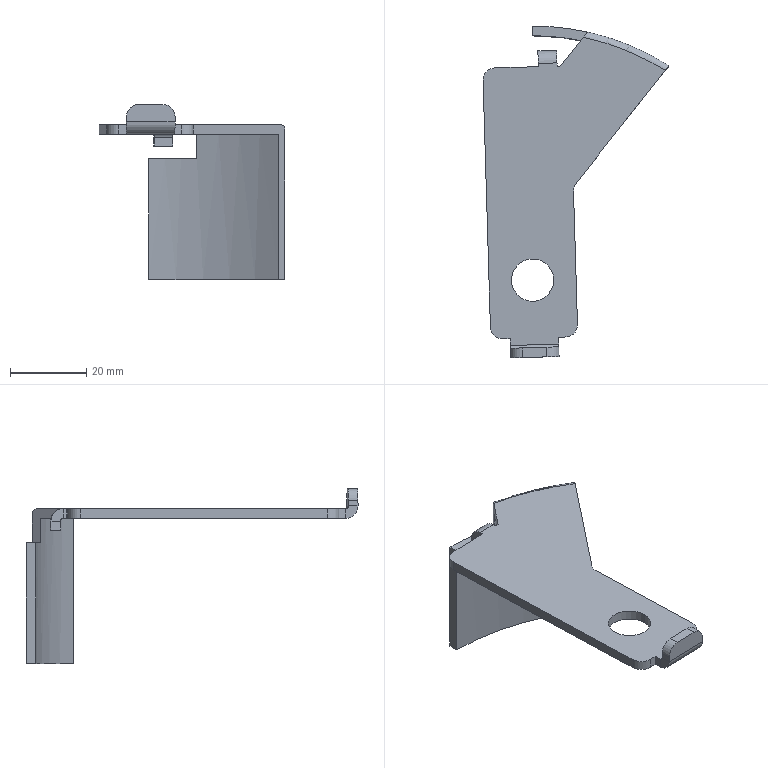Part | SolidWorks | features Fillet 2, ICE 2, SM3dBend 2, FlatPattern 1, SMBaseFlange 1, SheetMetal 1 | 1 solid | 47 faces | box 48.773 x 87.122 x 45.946 mm | volume 8989 mm3 | plane 31 | cylinder 15 | torus 1 | commonest cylinder face diameters 6.35 x7 1.473 x2 6.553 x2 11.112 x2 128.27 x1 133.35 x1
STEP:
#1=CARTESIAN_POINT('',(21.933,-23.71,2.54));
#2=VERTEX_POINT('',#1);
#3=CARTESIAN_POINT('',(21.935,-23.805,2.54));
#4=VERTEX_POINT('',#3);
#5=CARTESIAN_POINT('',(25.108,-23.71,2.54));
#6=DIRECTION('',(0.,0.,1.));
#7=DIRECTION('',(1.,0.,0.));
#8=AXIS2_PLACEMENT_3D('',#5,#6,#7);
#9=CIRCLE('',#8,3.175);
#10=EDGE_CURVE('',#2,#4,#9,.T.);
#11=ORIENTED_EDGE('',*,*,#10,.F.);
#12=CARTESIAN_POINT('',(21.933,-23.71,0.));
#13=VERTEX_POINT('',#12);
#14=CARTESIAN_POINT('',(21.933,-23.71,2.54));
#15=DIRECTION('',(0.,0.,-1.));
#16=VECTOR('',#15,1000.);
#17=LINE('',#14,#16);
#18=EDGE_CURVE('',#2,#13,#17,.T.);
#19=ORIENTED_EDGE('',*,*,#18,.T.);
#20=CARTESIAN_POINT('',(21.935,-23.805,0.));
#21=VERTEX_POINT('',#20);
#22=CARTESIAN_POINT('',(25.108,-23.71,0.));
#23=DIRECTION('',(0.,0.,-1.));
#24=DIRECTION('',(1.,0.,0.));
#25=AXIS2_PLACEMENT_3D('',#22,#23,#24);
#26=CIRCLE('',#25,3.175);
#27=EDGE_CURVE('',#21,#13,#26,.T.);
#28=ORIENTED_EDGE('',*,*,#27,.F.);
#29=CARTESIAN_POINT('',(21.935,-23.805,2.54));
#30=DIRECTION('',(0.,0.,-1.));
#31=VECTOR('',#30,1000.);
#32=LINE('',#29,#31);
#33=EDGE_CURVE('',#4,#21,#32,.T.);
#34=ORIENTED_EDGE('',*,*,#33,.F.);
#35=EDGE_LOOP('',(#11,#19,#28,#34));
#36=FACE_OUTER_BOUND('',#35,.T.);
#37=CARTESIAN_POINT('',(25.108,-23.71,2.54));
#38=DIRECTION('',(0.,0.,-1.));
#39=DIRECTION('',(-1.,0.,0.));
#40=AXIS2_PLACEMENT_3D('',#37,#38,#39);
#41=CYLINDRICAL_SURFACE('',#40,3.175);
#42=ADVANCED_FACE('',(#36),#41,.T.);
#43=CARTESIAN_POINT('',(29.369,-76.2,2.54));
#44=VERTEX_POINT('',#43);
#45=CARTESIAN_POINT('',(40.481,-76.2,2.54));
#46=VERTEX_POINT('',#45);
#47=CARTESIAN_POINT('',(34.925,-76.2,2.54));
#48=DIRECTION('',(0.,0.,1.));
#49=DIRECTION('',(1.,0.,0.));
#50=AXIS2_PLACEMENT_3D('',#47,#48,#49);
#51=CIRCLE('',#50,5.556);
#52=EDGE_CURVE('',#44,#46,#51,.T.);
#53=ORIENTED_EDGE('',*,*,#52,.T.);
#54=CARTESIAN_POINT('',(40.481,-76.2,0.));
#55=VERTEX_POINT('',#54);
#56=CARTESIAN_POINT('',(40.481,-76.2,2.54));
#57=DIRECTION('',(0.,0.,-1.));
#58=VECTOR('',#57,1000.);
#59=LINE('',#56,#58);
#60=EDGE_CURVE('',#46,#55,#59,.T.);
#61=ORIENTED_EDGE('',*,*,#60,.T.);
#62=CARTESIAN_POINT('',(29.369,-76.2,0.));
#63=VERTEX_POINT('',#62);
#64=CARTESIAN_POINT('',(34.925,-76.2,0.));
#65=DIRECTION('',(0.,0.,1.));
#66=DIRECTION('',(1.,0.,0.));
#67=AXIS2_PLACEMENT_3D('',#64,#65,#66);
#68=CIRCLE('',#67,5.556);
#69=EDGE_CURVE('',#63,#55,#68,.T.);
#70=ORIENTED_EDGE('',*,*,#69,.F.);
#71=CARTESIAN_POINT('',(29.369,-76.2,2.54));
#72=DIRECTION('',(0.,0.,-1.));
#73=VECTOR('',#72,1000.);
#74=LINE('',#71,#73);
#75=EDGE_CURVE('',#44,#63,#74,.T.);
#76=ORIENTED_EDGE('',*,*,#75,.F.);
#77=EDGE_LOOP('',(#53,#61,#70,#76));
#78=FACE_OUTER_BOUND('',#77,.T.);
#79=CARTESIAN_POINT('',(34.925,-76.2,2.54));
#80=DIRECTION('',(0.,0.,-1.));
#81=DIRECTION('',(-1.,0.,0.));
#82=AXIS2_PLACEMENT_3D('',#79,#80,#81);
#83=CYLINDRICAL_SURFACE('',#82,5.556);
#84=ADVANCED_FACE('',(#78),#83,.F.);
#85=CARTESIAN_POINT('',(48.266,-12.494,2.54));
#86=VERTEX_POINT('',#85);
#87=CARTESIAN_POINT('',(42.32,-20.023,2.54));
#88=VERTEX_POINT('',#87);
#89=CARTESIAN_POINT('',(49.362,-11.107,2.54));
#90=DIRECTION('',(-0.6198,-0.7848,0.));
#91=VECTOR('',#90,1000.);
#92=LINE('',#89,#91);
#93=EDGE_CURVE('',#86,#88,#92,.T.);
#94=ORIENTED_EDGE('',*,*,#93,.F.);
#95=CARTESIAN_POINT('',(49.362,-11.107,0.9525));
#96=VERTEX_POINT('',#95);
#97=CARTESIAN_POINT('',(48.266,-12.494,2.54));
#98=CARTESIAN_POINT('',(48.403,-12.32,2.54));
#99=CARTESIAN_POINT('',(48.537,-12.151,2.504));
#100=CARTESIAN_POINT('',(48.796,-11.823,2.357));
#101=CARTESIAN_POINT('',(48.914,-11.673,2.25));
#102=CARTESIAN_POINT('',(49.072,-11.474,2.034));
#103=CARTESIAN_POINT('',(49.119,-11.414,1.956));
#104=CARTESIAN_POINT('',(49.202,-11.308,1.784));
#105=CARTESIAN_POINT('',(49.239,-11.262,1.69));
#106=CARTESIAN_POINT('',(49.299,-11.185,1.492));
#107=CARTESIAN_POINT('',(49.322,-11.157,1.389));
#108=CARTESIAN_POINT('',(49.353,-11.117,1.175));
#109=CARTESIAN_POINT('',(49.362,-11.107,1.064));
#110=CARTESIAN_POINT('',(49.362,-11.107,0.9525));
#111=B_SPLINE_CURVE_WITH_KNOTS('',3,(#97,#98,#99,#100,#101,#102,#103,#104,#105,#106,#107,#108,#109,#110),.UNSPECIFIED.,.F.,.F.,(4,2,2,2,2,2,4),(0.,0.000656,0.001312,0.00164,0.001968,0.002296,0.002624),.UNSPECIFIED.);
#112=EDGE_CURVE('',#86,#96,#111,.T.);
#113=ORIENTED_EDGE('',*,*,#112,.T.);
#114=CARTESIAN_POINT('',(49.362,-11.107,-6.35));
#115=VERTEX_POINT('',#114);
#116=CARTESIAN_POINT('',(49.362,-11.107,2.54));
#117=DIRECTION('',(0.,0.,-1.));
#118=VECTOR('',#117,1000.);
#119=LINE('',#116,#118);
#120=EDGE_CURVE('',#96,#115,#119,.T.);
#121=ORIENTED_EDGE('',*,*,#120,.T.);
#122=CARTESIAN_POINT('',(47.605,-13.331,-6.35));
#123=VERTEX_POINT('',#122);
#124=CARTESIAN_POINT('',(49.362,-11.107,-6.35));
#125=DIRECTION('',(0.6198,0.7848,0.));
#126=VECTOR('',#125,1000.);
#127=LINE('',#124,#126);
#128=EDGE_CURVE('',#123,#115,#127,.T.);
#129=ORIENTED_EDGE('',*,*,#128,.F.);
#130=CARTESIAN_POINT('',(47.605,-13.331,0.));
#131=VERTEX_POINT('',#130);
#132=CARTESIAN_POINT('',(47.605,-13.331,-38.1));
#133=DIRECTION('',(0.,0.,1.));
#134=VECTOR('',#133,1000.);
#135=LINE('',#132,#134);
#136=EDGE_CURVE('',#123,#131,#135,.T.);
#137=ORIENTED_EDGE('',*,*,#136,.T.);
#138=CARTESIAN_POINT('',(42.32,-20.023,0.));
#139=VERTEX_POINT('',#138);
#140=CARTESIAN_POINT('',(49.362,-11.107,0.));
#141=DIRECTION('',(-0.6198,-0.7848,0.));
#142=VECTOR('',#141,1000.);
#143=LINE('',#140,#142);
#144=EDGE_CURVE('',#131,#139,#143,.T.);
#145=ORIENTED_EDGE('',*,*,#144,.T.);
#146=CARTESIAN_POINT('',(42.32,-20.023,2.54));
#147=DIRECTION('',(0.,0.,-1.));
#148=VECTOR('',#147,1000.);
#149=LINE('',#146,#148);
#150=EDGE_CURVE('',#88,#139,#149,.T.);
#151=ORIENTED_EDGE('',*,*,#150,.F.);
#152=EDGE_LOOP('',(#94,#113,#121,#129,#137,#145,#151));
#153=FACE_OUTER_BOUND('',#152,.T.);
#154=CARTESIAN_POINT('',(49.362,-11.107,2.54));
#155=DIRECTION('',(0.7848,-0.6198,0.));
#156=DIRECTION('',(0.6198,0.7848,0.));
#157=AXIS2_PLACEMENT_3D('',#154,#155,#156);
#158=PLANE('',#157);
#159=ADVANCED_FACE('',(#153),#158,.F.);
#160=ORIENTED_EDGE('',*,*,#69,.T.);
#161=CARTESIAN_POINT('',(34.925,-76.2,0.));
#162=DIRECTION('',(0.,0.,1.));
#163=DIRECTION('',(1.,0.,0.));
#164=AXIS2_PLACEMENT_3D('',#161,#162,#163);
#165=CIRCLE('',#164,5.556);
#166=EDGE_CURVE('',#55,#63,#165,.T.);
#167=ORIENTED_EDGE('',*,*,#166,.T.);
#168=EDGE_LOOP('',(#160,#167));
#169=FACE_BOUND('',#168,.T.);
#170=CARTESIAN_POINT('',(69.123,-21.943,0.));
#171=VERTEX_POINT('',#170);
#172=CARTESIAN_POINT('',(34.925,-76.2,0.));
#173=DIRECTION('',(0.,0.,1.));
#174=DIRECTION('',(-1.,0.,0.));
#175=AXIS2_PLACEMENT_3D('',#172,#173,#174);
#176=CIRCLE('',#175,64.135);
#177=EDGE_CURVE('',#171,#131,#176,.T.);
#178=ORIENTED_EDGE('',*,*,#177,.F.);
#179=CARTESIAN_POINT('',(46.349,-50.782,0.));
#180=VERTEX_POINT('',#179);
#181=CARTESIAN_POINT('',(45.632,-51.689,0.));
#182=DIRECTION('',(0.6198,0.7848,0.));
#183=VECTOR('',#182,1000.);
#184=LINE('',#181,#183);
#185=EDGE_CURVE('',#180,#171,#184,.T.);
#186=ORIENTED_EDGE('',*,*,#185,.F.);
#187=CARTESIAN_POINT('',(45.667,-52.844,0.));
#188=VERTEX_POINT('',#187);
#189=CARTESIAN_POINT('',(48.84,-52.75,0.));
#190=DIRECTION('',(0.,0.,1.));
#191=DIRECTION('',(1.,0.,0.));
#192=AXIS2_PLACEMENT_3D('',#189,#190,#191);
#193=CIRCLE('',#192,3.175);
#194=EDGE_CURVE('',#180,#188,#193,.T.);
#195=ORIENTED_EDGE('',*,*,#194,.T.);
#196=CARTESIAN_POINT('',(46.706,-87.868,0.));
#197=VERTEX_POINT('',#196);
#198=CARTESIAN_POINT('',(46.801,-91.041,0.));
#199=DIRECTION('',(-0.02967,0.9996,0.));
#200=VECTOR('',#199,1000.);
#201=LINE('',#198,#200);
#202=EDGE_CURVE('',#197,#188,#201,.T.);
#203=ORIENTED_EDGE('',*,*,#202,.F.);
#204=CARTESIAN_POINT('',(43.627,-91.136,0.));
#205=VERTEX_POINT('',#204);
#206=CARTESIAN_POINT('',(43.533,-87.962,0.));
#207=DIRECTION('',(0.,0.,-1.));
#208=DIRECTION('',(1.,0.,0.));
#209=AXIS2_PLACEMENT_3D('',#206,#207,#208);
#210=CIRCLE('',#209,3.175);
#211=EDGE_CURVE('',#197,#205,#210,.T.);
#212=ORIENTED_EDGE('',*,*,#211,.T.);
#213=CARTESIAN_POINT('',(41.723,-91.192,0.));
#214=VERTEX_POINT('',#213);
#215=CARTESIAN_POINT('',(41.723,-91.192,0.));
#216=DIRECTION('',(0.9996,0.02967,0.));
#217=VECTOR('',#216,1000.);
#218=LINE('',#215,#217);
#219=EDGE_CURVE('',#214,#205,#218,.T.);
#220=ORIENTED_EDGE('',*,*,#219,.F.);
#221=CARTESIAN_POINT('',(41.776,-92.995,0.));
#222=VERTEX_POINT('',#221);
#223=CARTESIAN_POINT('',(42.005,-100.713,0.));
#224=DIRECTION('',(-0.02967,0.9996,0.));
#225=VECTOR('',#224,1000.);
#226=LINE('',#223,#225);
#227=EDGE_CURVE('',#222,#214,#226,.T.);
#228=ORIENTED_EDGE('',*,*,#227,.F.);
#229=CARTESIAN_POINT('',(29.082,-93.371,0.));
#230=VERTEX_POINT('',#229);
#231=CARTESIAN_POINT('',(35.429,-93.183,0.));
#232=DIRECTION('',(-0.9996,-0.02967,0.));
#233=VECTOR('',#232,1000.);
#234=LINE('',#231,#233);
#235=EDGE_CURVE('',#222,#230,#234,.T.);
#236=ORIENTED_EDGE('',*,*,#235,.T.);
#237=CARTESIAN_POINT('',(29.028,-91.569,0.));
#238=VERTEX_POINT('',#237);
#239=CARTESIAN_POINT('',(29.028,-91.569,0.));
#240=DIRECTION('',(0.02967,-0.9996,0.));
#241=VECTOR('',#240,1000.);
#242=LINE('',#239,#241);
#243=EDGE_CURVE('',#238,#230,#242,.T.);
#244=ORIENTED_EDGE('',*,*,#243,.F.);
#245=CARTESIAN_POINT('',(27.124,-91.625,0.));
#246=VERTEX_POINT('',#245);
#247=CARTESIAN_POINT('',(23.951,-91.72,0.));
#248=DIRECTION('',(0.9996,0.02967,0.));
#249=VECTOR('',#248,1000.);
#250=LINE('',#247,#249);
#251=EDGE_CURVE('',#246,#238,#250,.T.);
#252=ORIENTED_EDGE('',*,*,#251,.F.);
#253=CARTESIAN_POINT('',(23.856,-88.546,0.));
#254=VERTEX_POINT('',#253);
#255=CARTESIAN_POINT('',(27.03,-88.452,0.));
#256=DIRECTION('',(0.,0.,-1.));
#257=DIRECTION('',(1.,0.,0.));
#258=AXIS2_PLACEMENT_3D('',#255,#256,#257);
#259=CIRCLE('',#258,3.175);
#260=EDGE_CURVE('',#246,#254,#259,.T.);
#261=ORIENTED_EDGE('',*,*,#260,.T.);
#262=CARTESIAN_POINT('',(21.84,-20.631,0.));
#263=DIRECTION('',(0.02967,-0.9996,0.));
#264=VECTOR('',#263,1000.);
#265=LINE('',#262,#264);
#266=EDGE_CURVE('',#21,#254,#265,.T.);
#267=ORIENTED_EDGE('',*,*,#266,.F.);
#268=ORIENTED_EDGE('',*,*,#27,.T.);
#269=CARTESIAN_POINT('',(25.014,-20.537,0.));
#270=VERTEX_POINT('',#269);
#271=CARTESIAN_POINT('',(25.108,-23.71,0.));
#272=DIRECTION('',(0.,0.,-1.));
#273=DIRECTION('',(1.,0.,0.));
#274=AXIS2_PLACEMENT_3D('',#271,#272,#273);
#275=CIRCLE('',#274,3.175);
#276=EDGE_CURVE('',#13,#270,#275,.T.);
#277=ORIENTED_EDGE('',*,*,#276,.T.);
#278=CARTESIAN_POINT('',(36.439,-20.198,0.));
#279=VERTEX_POINT('',#278);
#280=CARTESIAN_POINT('',(36.439,-20.198,0.));
#281=DIRECTION('',(-0.9996,-0.02967,0.));
#282=VECTOR('',#281,1000.);
#283=LINE('',#280,#282);
#284=EDGE_CURVE('',#279,#270,#283,.T.);
#285=ORIENTED_EDGE('',*,*,#284,.F.);
#286=CARTESIAN_POINT('',(36.414,-19.36,0.));
#287=VERTEX_POINT('',#286);
#288=CARTESIAN_POINT('',(36.25,-13.85,0.));
#289=DIRECTION('',(0.02967,-0.9996,0.));
#290=VECTOR('',#289,1000.);
#291=LINE('',#288,#290);
#292=EDGE_CURVE('',#287,#279,#291,.T.);
#293=ORIENTED_EDGE('',*,*,#292,.F.);
#294=CARTESIAN_POINT('',(41.328,-19.214,0.));
#295=VERTEX_POINT('',#294);
#296=CARTESIAN_POINT('',(33.24,-19.454,0.));
#297=DIRECTION('',(-0.9996,-0.02967,0.));
#298=VECTOR('',#297,1000.);
#299=LINE('',#296,#298);
#300=EDGE_CURVE('',#295,#287,#299,.T.);
#301=ORIENTED_EDGE('',*,*,#300,.F.);
#302=CARTESIAN_POINT('',(41.353,-20.052,0.));
#303=VERTEX_POINT('',#302);
#304=CARTESIAN_POINT('',(41.353,-20.052,0.));
#305=DIRECTION('',(-0.02967,0.9996,0.));
#306=VECTOR('',#305,1000.);
#307=LINE('',#304,#306);
#308=EDGE_CURVE('',#303,#295,#307,.T.);
#309=ORIENTED_EDGE('',*,*,#308,.F.);
#310=CARTESIAN_POINT('',(42.32,-20.023,0.));
#311=DIRECTION('',(-0.9996,-0.02967,0.));
#312=VECTOR('',#311,1000.);
#313=LINE('',#310,#312);
#314=EDGE_CURVE('',#139,#303,#313,.T.);
#315=ORIENTED_EDGE('',*,*,#314,.F.);
#316=ORIENTED_EDGE('',*,*,#144,.F.);
#317=EDGE_LOOP('',(#178,#186,#195,#203,#212,#220,#228,#236,#244,#252,#261,#267,#268,#277,#285,#293,#301,#309,#315,#316));
#318=FACE_OUTER_BOUND('',#317,.T.);
#319=CARTESIAN_POINT('',(34.925,-76.2,0.));
#320=DIRECTION('',(0.,0.,1.));
#321=DIRECTION('',(1.,0.,0.));
#322=AXIS2_PLACEMENT_3D('',#319,#320,#321);
#323=PLANE('',#322);
#324=ADVANCED_FACE('',(#169,#318),#323,.F.);
#325=ORIENTED_EDGE('',*,*,#243,.T.);
#326=CARTESIAN_POINT('',(29.082,-93.371,2.54));
#327=VERTEX_POINT('',#326);
#328=CARTESIAN_POINT('',(29.082,-93.371,2.54));
#329=DIRECTION('',(0.,0.,1.));
#330=VECTOR('',#329,1000.);
#331=LINE('',#328,#330);
#332=EDGE_CURVE('',#230,#327,#331,.T.);
#333=ORIENTED_EDGE('',*,*,#332,.T.);
#334=CARTESIAN_POINT('',(29.028,-91.569,2.54));
#335=VERTEX_POINT('',#334);
#336=CARTESIAN_POINT('',(29.028,-91.569,2.54));
#337=DIRECTION('',(0.02967,-0.9996,0.));
#338=VECTOR('',#337,1000.);
#339=LINE('',#336,#338);
#340=EDGE_CURVE('',#335,#327,#339,.T.);
#341=ORIENTED_EDGE('',*,*,#340,.F.);
#342=CARTESIAN_POINT('',(29.028,-91.569,2.54));
#343=DIRECTION('',(0.,0.,-1.));
#344=VECTOR('',#343,1000.);
#345=LINE('',#342,#344);
#346=EDGE_CURVE('',#335,#238,#345,.T.);
#347=ORIENTED_EDGE('',*,*,#346,.T.);
#348=EDGE_LOOP('',(#325,#333,#341,#347));
#349=FACE_OUTER_BOUND('',#348,.T.);
#350=CARTESIAN_POINT('',(29.028,-91.569,2.54));
#351=DIRECTION('',(0.9996,0.02967,0.));
#352=DIRECTION('',(-0.02967,0.9996,0.));
#353=AXIS2_PLACEMENT_3D('',#350,#351,#352);
#354=PLANE('',#353);
#355=ADVANCED_FACE('',(#349),#354,.F.);
#356=CARTESIAN_POINT('',(41.776,-92.995,2.54));
#357=VERTEX_POINT('',#356);
#358=CARTESIAN_POINT('',(41.723,-91.192,2.54));
#359=VERTEX_POINT('',#358);
#360=CARTESIAN_POINT('',(42.005,-100.713,2.54));
#361=DIRECTION('',(-0.02967,0.9996,0.));
#362=VECTOR('',#361,1000.);
#363=LINE('',#360,#362);
#364=EDGE_CURVE('',#357,#359,#363,.T.);
#365=ORIENTED_EDGE('',*,*,#364,.F.);
#366=CARTESIAN_POINT('',(41.776,-92.995,2.54));
#367=DIRECTION('',(0.,0.,-1.));
#368=VECTOR('',#367,1000.);
#369=LINE('',#366,#368);
#370=EDGE_CURVE('',#357,#222,#369,.T.);
#371=ORIENTED_EDGE('',*,*,#370,.T.);
#372=ORIENTED_EDGE('',*,*,#227,.T.);
#373=CARTESIAN_POINT('',(41.723,-91.192,2.54));
#374=DIRECTION('',(0.,0.,-1.));
#375=VECTOR('',#374,1000.);
#376=LINE('',#373,#375);
#377=EDGE_CURVE('',#359,#214,#376,.T.);
#378=ORIENTED_EDGE('',*,*,#377,.F.);
#379=EDGE_LOOP('',(#365,#371,#372,#378));
#380=FACE_OUTER_BOUND('',#379,.T.);
#381=CARTESIAN_POINT('',(42.005,-100.713,2.54));
#382=DIRECTION('',(-0.9996,-0.02967,0.));
#383=DIRECTION('',(0.02967,-0.9996,0.));
#384=AXIS2_PLACEMENT_3D('',#381,#382,#383);
#385=PLANE('',#384);
#386=ADVANCED_FACE('',(#380),#385,.F.);
#387=CARTESIAN_POINT('',(41.306,-18.478,-0.7366));
#388=VERTEX_POINT('',#387);
#389=CARTESIAN_POINT('',(41.306,-18.478,-3.096));
#390=VERTEX_POINT('',#389);
#391=CARTESIAN_POINT('',(41.306,-18.478,3.254));
#392=DIRECTION('',(0.,0.,-1.));
#393=VECTOR('',#392,1000.);
#394=LINE('',#391,#393);
#395=EDGE_CURVE('',#388,#390,#394,.T.);
#396=ORIENTED_EDGE('',*,*,#395,.F.);
#397=CARTESIAN_POINT('',(36.392,-18.623,-0.7366));
#398=VERTEX_POINT('',#397);
#399=CARTESIAN_POINT('',(33.219,-18.718,-0.7366));
#400=DIRECTION('',(-0.9996,-0.02967,0.));
#401=VECTOR('',#400,1000.);
#402=LINE('',#399,#401);
#403=EDGE_CURVE('',#388,#398,#402,.T.);
#404=ORIENTED_EDGE('',*,*,#403,.T.);
#405=CARTESIAN_POINT('',(36.392,-18.623,-3.096));
#406=VERTEX_POINT('',#405);
#407=CARTESIAN_POINT('',(36.392,-18.623,-3.096));
#408=DIRECTION('',(0.,0.,1.));
#409=VECTOR('',#408,1000.);
#410=LINE('',#407,#409);
#411=EDGE_CURVE('',#406,#398,#410,.T.);
#412=ORIENTED_EDGE('',*,*,#411,.F.);
#413=CARTESIAN_POINT('',(41.306,-18.478,-3.096));
#414=DIRECTION('',(-0.9996,-0.02967,0.));
#415=VECTOR('',#414,1000.);
#416=LINE('',#413,#415);
#417=EDGE_CURVE('',#390,#406,#416,.T.);
#418=ORIENTED_EDGE('',*,*,#417,.F.);
#419=EDGE_LOOP('',(#396,#404,#412,#418));
#420=FACE_OUTER_BOUND('',#419,.T.);
#421=CARTESIAN_POINT('',(33.219,-18.718,59.186));
#422=DIRECTION('',(-0.02967,0.9996,0.));
#423=DIRECTION('',(0.9991,0.02966,0.02967));
#424=AXIS2_PLACEMENT_3D('',#421,#422,#423);
#425=PLANE('',#424);
#426=ADVANCED_FACE('',(#420),#425,.F.);
#427=CARTESIAN_POINT('',(41.23,-15.939,-0.7366));
#428=VERTEX_POINT('',#427);
#429=CARTESIAN_POINT('',(41.23,-15.939,-3.096));
#430=VERTEX_POINT('',#429);
#431=CARTESIAN_POINT('',(41.23,-15.939,3.254));
#432=DIRECTION('',(0.,0.,-1.));
#433=VECTOR('',#432,1000.);
#434=LINE('',#431,#433);
#435=EDGE_CURVE('',#428,#430,#434,.T.);
#436=ORIENTED_EDGE('',*,*,#435,.F.);
#437=CARTESIAN_POINT('',(41.23,-15.939,-0.7366));
#438=DIRECTION('',(0.02967,-0.9996,0.));
#439=VECTOR('',#438,1000.);
#440=LINE('',#437,#439);
#441=EDGE_CURVE('',#428,#388,#440,.T.);
#442=ORIENTED_EDGE('',*,*,#441,.T.);
#443=ORIENTED_EDGE('',*,*,#395,.T.);
#444=CARTESIAN_POINT('',(41.23,-15.939,-3.096));
#445=DIRECTION('',(0.02967,-0.9996,0.));
#446=VECTOR('',#445,1000.);
#447=LINE('',#444,#446);
#448=EDGE_CURVE('',#430,#390,#447,.T.);
#449=ORIENTED_EDGE('',*,*,#448,.F.);
#450=EDGE_LOOP('',(#436,#442,#443,#449));
#451=FACE_OUTER_BOUND('',#450,.T.);
#452=CARTESIAN_POINT('',(41.23,-15.939,3.254));
#453=DIRECTION('',(-0.9996,-0.02967,0.));
#454=DIRECTION('',(0.,0.,1.));
#455=AXIS2_PLACEMENT_3D('',#452,#453,#454);
#456=PLANE('',#455);
#457=ADVANCED_FACE('',(#451),#456,.F.);
#458=ORIENTED_EDGE('',*,*,#411,.T.);
#459=CARTESIAN_POINT('',(36.317,-16.085,-0.7366));
#460=VERTEX_POINT('',#459);
#461=CARTESIAN_POINT('',(36.317,-16.085,-0.7366));
#462=DIRECTION('',(-0.02967,0.9996,0.));
#463=VECTOR('',#462,1000.);
#464=LINE('',#461,#463);
#465=EDGE_CURVE('',#398,#460,#464,.T.);
#466=ORIENTED_EDGE('',*,*,#465,.T.);
#467=CARTESIAN_POINT('',(36.317,-16.085,-3.096));
#468=VERTEX_POINT('',#467);
#469=CARTESIAN_POINT('',(36.317,-16.085,-3.096));
#470=DIRECTION('',(0.,0.,1.));
#471=VECTOR('',#470,1000.);
#472=LINE('',#469,#471);
#473=EDGE_CURVE('',#468,#460,#472,.T.);
#474=ORIENTED_EDGE('',*,*,#473,.F.);
#475=CARTESIAN_POINT('',(36.317,-16.085,-3.096));
#476=DIRECTION('',(0.02967,-0.9996,0.));
#477=VECTOR('',#476,1000.);
#478=LINE('',#475,#477);
#479=EDGE_CURVE('',#468,#406,#478,.T.);
#480=ORIENTED_EDGE('',*,*,#479,.T.);
#481=EDGE_LOOP('',(#458,#466,#474,#480));
#482=FACE_OUTER_BOUND('',#481,.T.);
#483=CARTESIAN_POINT('',(36.317,-16.085,-3.096));
#484=DIRECTION('',(0.9996,0.02967,0.));
#485=DIRECTION('',(0.,0.,-1.));
#486=AXIS2_PLACEMENT_3D('',#483,#484,#485);
#487=PLANE('',#486);
#488=ADVANCED_FACE('',(#482),#487,.F.);
#489=CARTESIAN_POINT('',(33.143,-16.179,-0.7366));
#490=DIRECTION('',(-0.9996,-0.02967,0.));
#491=VECTOR('',#490,1000.);
#492=LINE('',#489,#491);
#493=EDGE_CURVE('',#428,#460,#492,.T.);
#494=ORIENTED_EDGE('',*,*,#493,.F.);
#495=ORIENTED_EDGE('',*,*,#435,.T.);
#496=CARTESIAN_POINT('',(41.23,-15.939,-3.096));
#497=DIRECTION('',(-0.9996,-0.02967,0.));
#498=VECTOR('',#497,1000.);
#499=LINE('',#496,#498);
#500=EDGE_CURVE('',#430,#468,#499,.T.);
#501=ORIENTED_EDGE('',*,*,#500,.T.);
#502=ORIENTED_EDGE('',*,*,#473,.T.);
#503=EDGE_LOOP('',(#494,#495,#501,#502));
#504=FACE_OUTER_BOUND('',#503,.T.);
#505=CARTESIAN_POINT('',(33.143,-16.179,59.186));
#506=DIRECTION('',(-0.02967,0.9996,0.));
#507=DIRECTION('',(0.9991,0.02966,0.02967));
#508=AXIS2_PLACEMENT_3D('',#505,#506,#507);
#509=PLANE('',#508);
#510=ADVANCED_FACE('',(#504),#509,.T.);
#511=ORIENTED_EDGE('',*,*,#417,.T.);
#512=ORIENTED_EDGE('',*,*,#479,.F.);
#513=ORIENTED_EDGE('',*,*,#500,.F.);
#514=ORIENTED_EDGE('',*,*,#448,.T.);
#515=EDGE_LOOP('',(#511,#512,#513,#514));
#516=FACE_OUTER_BOUND('',#515,.T.);
#517=CARTESIAN_POINT('',(41.23,-15.939,-3.096));
#518=DIRECTION('',(0.,0.,1.));
#519=DIRECTION('',(0.9996,0.02967,0.));
#520=AXIS2_PLACEMENT_3D('',#517,#518,#519);
#521=PLANE('',#520);
#522=ADVANCED_FACE('',(#516),#521,.F.);
#523=ORIENTED_EDGE('',*,*,#314,.T.);
#524=CARTESIAN_POINT('',(41.353,-20.052,2.54));
#525=VERTEX_POINT('',#524);
#526=CARTESIAN_POINT('',(41.353,-20.052,2.54));
#527=DIRECTION('',(0.,0.,-1.));
#528=VECTOR('',#527,1000.);
#529=LINE('',#526,#528);
#530=EDGE_CURVE('',#525,#303,#529,.T.);
#531=ORIENTED_EDGE('',*,*,#530,.F.);
#532=CARTESIAN_POINT('',(42.32,-20.023,2.54));
#533=DIRECTION('',(-0.9996,-0.02967,0.));
#534=VECTOR('',#533,1000.);
#535=LINE('',#532,#534);
#536=EDGE_CURVE('',#88,#525,#535,.T.);
#537=ORIENTED_EDGE('',*,*,#536,.F.);
#538=ORIENTED_EDGE('',*,*,#150,.T.);
#539=EDGE_LOOP('',(#523,#531,#537,#538));
#540=FACE_OUTER_BOUND('',#539,.T.);
#541=CARTESIAN_POINT('',(42.32,-20.023,2.54));
#542=DIRECTION('',(0.02967,-0.9996,0.));
#543=DIRECTION('',(0.9996,0.02967,0.));
#544=AXIS2_PLACEMENT_3D('',#541,#542,#543);
#545=PLANE('',#544);
#546=ADVANCED_FACE('',(#540),#545,.F.);
#547=ORIENTED_EDGE('',*,*,#120,.F.);
#548=CARTESIAN_POINT('',(70.706,-19.939,0.9525));
#549=VERTEX_POINT('',#548);
#550=CARTESIAN_POINT('',(34.925,-76.2,0.9525));
#551=DIRECTION('',(0.,0.,-1.));
#552=DIRECTION('',(1.,0.,0.));
#553=AXIS2_PLACEMENT_3D('',#550,#551,#552);
#554=CIRCLE('',#553,66.675);
#555=EDGE_CURVE('',#96,#549,#554,.T.);
#556=ORIENTED_EDGE('',*,*,#555,.T.);
#557=CARTESIAN_POINT('',(70.706,-19.939,-38.1));
#558=VERTEX_POINT('',#557);
#559=CARTESIAN_POINT('',(70.706,-19.939,2.54));
#560=DIRECTION('',(0.,0.,-1.));
#561=VECTOR('',#560,1000.);
#562=LINE('',#559,#561);
#563=EDGE_CURVE('',#549,#558,#562,.T.);
#564=ORIENTED_EDGE('',*,*,#563,.T.);
#565=CARTESIAN_POINT('',(34.925,-9.525,-38.1));
#566=VERTEX_POINT('',#565);
#567=CARTESIAN_POINT('',(34.925,-76.2,-38.1));
#568=DIRECTION('',(0.,0.,-1.));
#569=DIRECTION('',(-1.,0.,0.));
#570=AXIS2_PLACEMENT_3D('',#567,#568,#569);
#571=CIRCLE('',#570,66.675);
#572=EDGE_CURVE('',#566,#558,#571,.T.);
#573=ORIENTED_EDGE('',*,*,#572,.F.);
#574=CARTESIAN_POINT('',(34.925,-9.525,-6.35));
#575=VERTEX_POINT('',#574);
#576=CARTESIAN_POINT('',(34.925,-9.525,-6.35));
#577=DIRECTION('',(0.,0.,-1.));
#578=VECTOR('',#577,1000.);
#579=LINE('',#576,#578);
#580=EDGE_CURVE('',#575,#566,#579,.T.);
#581=ORIENTED_EDGE('',*,*,#580,.F.);
#582=CARTESIAN_POINT('',(34.925,-76.2,-6.35));
#583=DIRECTION('',(0.,0.,-1.));
#584=DIRECTION('',(-1.,0.,0.));
#585=AXIS2_PLACEMENT_3D('',#582,#583,#584);
#586=CIRCLE('',#585,66.675);
#587=EDGE_CURVE('',#575,#115,#586,.T.);
#588=ORIENTED_EDGE('',*,*,#587,.T.);
#589=EDGE_LOOP('',(#547,#556,#564,#573,#581,#588));
#590=FACE_OUTER_BOUND('',#589,.T.);
#591=CARTESIAN_POINT('',(34.925,-76.2,2.54));
#592=DIRECTION('',(0.,0.,-1.));
#593=DIRECTION('',(-1.,0.,0.));
#594=AXIS2_PLACEMENT_3D('',#591,#592,#593);
#595=CYLINDRICAL_SURFACE('',#594,66.675);
#596=ADVANCED_FACE('',(#590),#595,.T.);
#597=ORIENTED_EDGE('',*,*,#563,.F.);
#598=CARTESIAN_POINT('',(69.717,-21.192,2.54));
#599=VERTEX_POINT('',#598);
#600=CARTESIAN_POINT('',(70.706,-19.939,0.9525));
#601=CARTESIAN_POINT('',(70.706,-19.939,1.058));
#602=CARTESIAN_POINT('',(70.7,-19.947,1.161));
#603=CARTESIAN_POINT('',(70.674,-19.979,1.364));
#604=CARTESIAN_POINT('',(70.655,-20.004,1.465));
#605=CARTESIAN_POINT('',(70.606,-20.067,1.658));
#606=CARTESIAN_POINT('',(70.575,-20.105,1.749));
#607=CARTESIAN_POINT('',(70.503,-20.196,1.921));
#608=CARTESIAN_POINT('',(70.461,-20.249,2.003));
#609=CARTESIAN_POINT('',(70.324,-20.423,2.222));
#610=CARTESIAN_POINT('',(70.214,-20.562,2.34));
#611=CARTESIAN_POINT('',(69.977,-20.863,2.498));
#612=CARTESIAN_POINT('',(69.847,-21.027,2.54));
#613=CARTESIAN_POINT('',(69.717,-21.192,2.54));
#614=B_SPLINE_CURVE_WITH_KNOTS('',3,(#600,#601,#602,#603,#604,#605,#606,#607,#608,#609,#610,#611,#612,#613),.UNSPECIFIED.,.F.,.F.,(4,2,2,2,2,2,4),(0.,0.0003108,0.0006216,0.0009325,0.001243,0.001865,0.002487),.UNSPECIFIED.);
#615=EDGE_CURVE('',#549,#599,#614,.T.);
#616=ORIENTED_EDGE('',*,*,#615,.T.);
#617=CARTESIAN_POINT('',(46.349,-50.782,2.54));
#618=VERTEX_POINT('',#617);
#619=CARTESIAN_POINT('',(45.632,-51.689,2.54));
#620=DIRECTION('',(0.6198,0.7848,0.));
#621=VECTOR('',#620,1000.);
#622=LINE('',#619,#621);
#623=EDGE_CURVE('',#618,#599,#622,.T.);
#624=ORIENTED_EDGE('',*,*,#623,.F.);
#625=CARTESIAN_POINT('',(46.349,-50.782,0.));
#626=DIRECTION('',(0.,0.,-1.));
#627=VECTOR('',#626,1000.);
#628=LINE('',#625,#627);
#629=EDGE_CURVE('',#618,#180,#628,.T.);
#630=ORIENTED_EDGE('',*,*,#629,.T.);
#631=ORIENTED_EDGE('',*,*,#185,.T.);
#632=CARTESIAN_POINT('',(69.123,-21.943,-38.1));
#633=VERTEX_POINT('',#632);
#634=CARTESIAN_POINT('',(69.123,-21.943,-38.1));
#635=DIRECTION('',(0.,0.,1.));
#636=VECTOR('',#635,1000.);
#637=LINE('',#634,#636);
#638=EDGE_CURVE('',#633,#171,#637,.T.);
#639=ORIENTED_EDGE('',*,*,#638,.F.);
#640=CARTESIAN_POINT('',(69.123,-21.943,-38.1));
#641=DIRECTION('',(-0.6198,-0.7848,0.));
#642=VECTOR('',#641,1000.);
#643=LINE('',#640,#642);
#644=EDGE_CURVE('',#558,#633,#643,.T.);
#645=ORIENTED_EDGE('',*,*,#644,.F.);
#646=EDGE_LOOP('',(#597,#616,#624,#630,#631,#639,#645));
#647=FACE_OUTER_BOUND('',#646,.T.);
#648=CARTESIAN_POINT('',(45.632,-51.689,2.54));
#649=DIRECTION('',(-0.7848,0.6198,0.));
#650=DIRECTION('',(-0.6198,-0.7848,0.));
#651=AXIS2_PLACEMENT_3D('',#648,#649,#650);
#652=PLANE('',#651);
#653=ADVANCED_FACE('',(#647),#652,.F.);
#654=ORIENTED_EDGE('',*,*,#202,.T.);
#655=CARTESIAN_POINT('',(45.667,-52.844,2.54));
#656=VERTEX_POINT('',#655);
#657=CARTESIAN_POINT('',(45.667,-52.844,2.54));
#658=DIRECTION('',(0.,0.,1.));
#659=VECTOR('',#658,1000.);
#660=LINE('',#657,#659);
#661=EDGE_CURVE('',#188,#656,#660,.T.);
#662=ORIENTED_EDGE('',*,*,#661,.T.);
#663=CARTESIAN_POINT('',(46.706,-87.868,2.54));
#664=VERTEX_POINT('',#663);
#665=CARTESIAN_POINT('',(46.801,-91.041,2.54));
#666=DIRECTION('',(-0.02967,0.9996,0.));
#667=VECTOR('',#666,1000.);
#668=LINE('',#665,#667);
#669=EDGE_CURVE('',#664,#656,#668,.T.);
#670=ORIENTED_EDGE('',*,*,#669,.F.);
#671=CARTESIAN_POINT('',(46.706,-87.868,2.54));
#672=DIRECTION('',(0.,0.,-1.));
#673=VECTOR('',#672,1000.);
#674=LINE('',#671,#673);
#675=EDGE_CURVE('',#664,#197,#674,.T.);
#676=ORIENTED_EDGE('',*,*,#675,.T.);
#677=EDGE_LOOP('',(#654,#662,#670,#676));
#678=FACE_OUTER_BOUND('',#677,.T.);
#679=CARTESIAN_POINT('',(46.801,-91.041,2.54));
#680=DIRECTION('',(-0.9996,-0.02967,0.));
#681=DIRECTION('',(0.02967,-0.9996,0.));
#682=AXIS2_PLACEMENT_3D('',#679,#680,#681);
#683=PLANE('',#682);
#684=ADVANCED_FACE('',(#678),#683,.F.);
#685=ORIENTED_EDGE('',*,*,#219,.T.);
#686=CARTESIAN_POINT('',(43.627,-91.136,2.54));
#687=VERTEX_POINT('',#686);
#688=CARTESIAN_POINT('',(43.627,-91.136,2.54));
#689=DIRECTION('',(0.,0.,1.));
#690=VECTOR('',#689,1000.);
#691=LINE('',#688,#690);
#692=EDGE_CURVE('',#205,#687,#691,.T.);
#693=ORIENTED_EDGE('',*,*,#692,.T.);
#694=CARTESIAN_POINT('',(41.723,-91.192,2.54));
#695=DIRECTION('',(0.9996,0.02967,0.));
#696=VECTOR('',#695,1000.);
#697=LINE('',#694,#696);
#698=EDGE_CURVE('',#359,#687,#697,.T.);
#699=ORIENTED_EDGE('',*,*,#698,.F.);
#700=ORIENTED_EDGE('',*,*,#377,.T.);
#701=EDGE_LOOP('',(#685,#693,#699,#700));
#702=FACE_OUTER_BOUND('',#701,.T.);
#703=CARTESIAN_POINT('',(41.723,-91.192,2.54));
#704=DIRECTION('',(-0.02967,0.9996,0.));
#705=DIRECTION('',(-0.9996,-0.02967,0.));
#706=AXIS2_PLACEMENT_3D('',#703,#704,#705);
#707=PLANE('',#706);
#708=ADVANCED_FACE('',(#702),#707,.F.);
#709=CARTESIAN_POINT('',(27.124,-91.625,2.54));
#710=VERTEX_POINT('',#709);
#711=CARTESIAN_POINT('',(23.951,-91.72,2.54));
#712=DIRECTION('',(0.9996,0.02967,0.));
#713=VECTOR('',#712,1000.);
#714=LINE('',#711,#713);
#715=EDGE_CURVE('',#710,#335,#714,.T.);
#716=ORIENTED_EDGE('',*,*,#715,.F.);
#717=CARTESIAN_POINT('',(27.124,-91.625,2.54));
#718=DIRECTION('',(0.,0.,-1.));
#719=VECTOR('',#718,1000.);
#720=LINE('',#717,#719);
#721=EDGE_CURVE('',#710,#246,#720,.T.);
#722=ORIENTED_EDGE('',*,*,#721,.T.);
#723=ORIENTED_EDGE('',*,*,#251,.T.);
#724=ORIENTED_EDGE('',*,*,#346,.F.);
#725=EDGE_LOOP('',(#716,#722,#723,#724));
#726=FACE_OUTER_BOUND('',#725,.T.);
#727=CARTESIAN_POINT('',(23.951,-91.72,2.54));
#728=DIRECTION('',(-0.02967,0.9996,0.));
#729=DIRECTION('',(-0.9996,-0.02967,0.));
#730=AXIS2_PLACEMENT_3D('',#727,#728,#729);
#731=PLANE('',#730);
#732=ADVANCED_FACE('',(#726),#731,.F.);
#733=ORIENTED_EDGE('',*,*,#266,.T.);
#734=CARTESIAN_POINT('',(23.856,-88.546,2.54));
#735=VERTEX_POINT('',#734);
#736=CARTESIAN_POINT('',(23.856,-88.546,2.54));
#737=DIRECTION('',(0.,0.,1.));
#738=VECTOR('',#737,1000.);
#739=LINE('',#736,#738);
#740=EDGE_CURVE('',#254,#735,#739,.T.);
#741=ORIENTED_EDGE('',*,*,#740,.T.);
#742=CARTESIAN_POINT('',(21.84,-20.631,2.54));
#743=DIRECTION('',(0.02967,-0.9996,0.));
#744=VECTOR('',#743,1000.);
#745=LINE('',#742,#744);
#746=EDGE_CURVE('',#4,#735,#745,.T.);
#747=ORIENTED_EDGE('',*,*,#746,.F.);
#748=ORIENTED_EDGE('',*,*,#33,.T.);
#749=EDGE_LOOP('',(#733,#741,#747,#748));
#750=FACE_OUTER_BOUND('',#749,.T.);
#751=CARTESIAN_POINT('',(21.84,-20.631,2.54));
#752=DIRECTION('',(0.9996,0.02967,0.));
#753=DIRECTION('',(-0.02967,0.9996,0.));
#754=AXIS2_PLACEMENT_3D('',#751,#752,#753);
#755=PLANE('',#754);
#756=ADVANCED_FACE('',(#750),#755,.F.);
#757=ORIENTED_EDGE('',*,*,#284,.T.);
#758=CARTESIAN_POINT('',(25.014,-20.537,2.54));
#759=VERTEX_POINT('',#758);
#760=CARTESIAN_POINT('',(25.014,-20.537,2.54));
#761=DIRECTION('',(0.,0.,1.));
#762=VECTOR('',#761,1000.);
#763=LINE('',#760,#762);
#764=EDGE_CURVE('',#270,#759,#763,.T.);
#765=ORIENTED_EDGE('',*,*,#764,.T.);
#766=CARTESIAN_POINT('',(36.439,-20.198,2.54));
#767=VERTEX_POINT('',#766);
#768=CARTESIAN_POINT('',(36.439,-20.198,2.54));
#769=DIRECTION('',(-0.9996,-0.02967,0.));
#770=VECTOR('',#769,1000.);
#771=LINE('',#768,#770);
#772=EDGE_CURVE('',#767,#759,#771,.T.);
#773=ORIENTED_EDGE('',*,*,#772,.F.);
#774=CARTESIAN_POINT('',(36.439,-20.198,2.54));
#775=DIRECTION('',(0.,0.,-1.));
#776=VECTOR('',#775,1000.);
#777=LINE('',#774,#776);
#778=EDGE_CURVE('',#767,#279,#777,.T.);
#779=ORIENTED_EDGE('',*,*,#778,.T.);
#780=EDGE_LOOP('',(#757,#765,#773,#779));
#781=FACE_OUTER_BOUND('',#780,.T.);
#782=CARTESIAN_POINT('',(36.439,-20.198,2.54));
#783=DIRECTION('',(0.02967,-0.9996,0.));
#784=DIRECTION('',(0.9996,0.02967,0.));
#785=AXIS2_PLACEMENT_3D('',#782,#783,#784);
#786=PLANE('',#785);
#787=ADVANCED_FACE('',(#781),#786,.F.);
#788=ORIENTED_EDGE('',*,*,#60,.F.);
#789=CARTESIAN_POINT('',(34.925,-76.2,2.54));
#790=DIRECTION('',(0.,0.,1.));
#791=DIRECTION('',(1.,0.,0.));
#792=AXIS2_PLACEMENT_3D('',#789,#790,#791);
#793=CIRCLE('',#792,5.556);
#794=EDGE_CURVE('',#46,#44,#793,.T.);
#795=ORIENTED_EDGE('',*,*,#794,.T.);
#796=ORIENTED_EDGE('',*,*,#75,.T.);
#797=ORIENTED_EDGE('',*,*,#166,.F.);
#798=EDGE_LOOP('',(#788,#795,#796,#797));
#799=FACE_OUTER_BOUND('',#798,.T.);
#800=CARTESIAN_POINT('',(34.925,-76.2,2.54));
#801=DIRECTION('',(0.,0.,-1.));
#802=DIRECTION('',(-1.,0.,0.));
#803=AXIS2_PLACEMENT_3D('',#800,#801,#802);
#804=CYLINDRICAL_SURFACE('',#803,5.556);
#805=ADVANCED_FACE('',(#799),#804,.F.);
#806=ORIENTED_EDGE('',*,*,#623,.T.);
#807=CARTESIAN_POINT('',(34.925,-76.2,2.54));
#808=DIRECTION('',(0.,0.,1.));
#809=DIRECTION('',(1.,0.,0.));
#810=AXIS2_PLACEMENT_3D('',#807,#808,#809);
#811=CIRCLE('',#810,65.087);
#812=EDGE_CURVE('',#599,#86,#811,.T.);
#813=ORIENTED_EDGE('',*,*,#812,.T.);
#814=ORIENTED_EDGE('',*,*,#93,.T.);
#815=ORIENTED_EDGE('',*,*,#536,.T.);
#816=CARTESIAN_POINT('',(41.328,-19.214,2.54));
#817=VERTEX_POINT('',#816);
#818=CARTESIAN_POINT('',(41.353,-20.052,2.54));
#819=DIRECTION('',(-0.02967,0.9996,0.));
#820=VECTOR('',#819,1000.);
#821=LINE('',#818,#820);
#822=EDGE_CURVE('',#525,#817,#821,.T.);
#823=ORIENTED_EDGE('',*,*,#822,.T.);
#824=CARTESIAN_POINT('',(36.414,-19.36,2.54));
#825=VERTEX_POINT('',#824);
#826=CARTESIAN_POINT('',(33.24,-19.454,2.54));
#827=DIRECTION('',(-0.9996,-0.02967,0.));
#828=VECTOR('',#827,1000.);
#829=LINE('',#826,#828);
#830=EDGE_CURVE('',#817,#825,#829,.T.);
#831=ORIENTED_EDGE('',*,*,#830,.T.);
#832=CARTESIAN_POINT('',(36.25,-13.85,2.54));
#833=DIRECTION('',(0.02967,-0.9996,0.));
#834=VECTOR('',#833,1000.);
#835=LINE('',#832,#834);
#836=EDGE_CURVE('',#825,#767,#835,.T.);
#837=ORIENTED_EDGE('',*,*,#836,.T.);
#838=ORIENTED_EDGE('',*,*,#772,.T.);
#839=CARTESIAN_POINT('',(25.108,-23.71,2.54));
#840=DIRECTION('',(0.,0.,1.));
#841=DIRECTION('',(1.,0.,0.));
#842=AXIS2_PLACEMENT_3D('',#839,#840,#841);
#843=CIRCLE('',#842,3.175);
#844=EDGE_CURVE('',#759,#2,#843,.T.);
#845=ORIENTED_EDGE('',*,*,#844,.T.);
#846=ORIENTED_EDGE('',*,*,#10,.T.);
#847=ORIENTED_EDGE('',*,*,#746,.T.);
#848=CARTESIAN_POINT('',(27.03,-88.452,2.54));
#849=DIRECTION('',(0.,0.,1.));
#850=DIRECTION('',(1.,0.,0.));
#851=AXIS2_PLACEMENT_3D('',#848,#849,#850);
#852=CIRCLE('',#851,3.175);
#853=EDGE_CURVE('',#735,#710,#852,.T.);
#854=ORIENTED_EDGE('',*,*,#853,.T.);
#855=ORIENTED_EDGE('',*,*,#715,.T.);
#856=ORIENTED_EDGE('',*,*,#340,.T.);
#857=CARTESIAN_POINT('',(35.429,-93.183,2.54));
#858=DIRECTION('',(-0.9996,-0.02967,0.));
#859=VECTOR('',#858,1000.);
#860=LINE('',#857,#859);
#861=EDGE_CURVE('',#357,#327,#860,.T.);
#862=ORIENTED_EDGE('',*,*,#861,.F.);
#863=ORIENTED_EDGE('',*,*,#364,.T.);
#864=ORIENTED_EDGE('',*,*,#698,.T.);
#865=CARTESIAN_POINT('',(43.533,-87.962,2.54));
#866=DIRECTION('',(0.,0.,1.));
#867=DIRECTION('',(1.,0.,0.));
#868=AXIS2_PLACEMENT_3D('',#865,#866,#867);
#869=CIRCLE('',#868,3.175);
#870=EDGE_CURVE('',#687,#664,#869,.T.);
#871=ORIENTED_EDGE('',*,*,#870,.T.);
#872=ORIENTED_EDGE('',*,*,#669,.T.);
#873=CARTESIAN_POINT('',(48.84,-52.75,2.54));
#874=DIRECTION('',(0.,0.,-1.));
#875=DIRECTION('',(1.,0.,0.));
#876=AXIS2_PLACEMENT_3D('',#873,#874,#875);
#877=CIRCLE('',#876,3.175);
#878=EDGE_CURVE('',#656,#618,#877,.T.);
#879=ORIENTED_EDGE('',*,*,#878,.T.);
#880=EDGE_LOOP('',(#806,#813,#814,#815,#823,#831,#837,#838,#845,#846,#847,#854,#855,#856,#862,#863,#864,#871,#872,#879));
#881=FACE_OUTER_BOUND('',#880,.T.);
#882=ORIENTED_EDGE('',*,*,#52,.F.);
#883=ORIENTED_EDGE('',*,*,#794,.F.);
#884=EDGE_LOOP('',(#882,#883));
#885=FACE_BOUND('',#884,.T.);
#886=CARTESIAN_POINT('',(34.925,-76.2,2.54));
#887=DIRECTION('',(0.,0.,1.));
#888=DIRECTION('',(1.,0.,0.));
#889=AXIS2_PLACEMENT_3D('',#886,#887,#888);
#890=PLANE('',#889);
#891=ADVANCED_FACE('',(#881,#885),#890,.T.);
#892=CARTESIAN_POINT('',(36.414,-19.36,2.54));
#893=DIRECTION('',(0.,0.,1.));
#894=VECTOR('',#893,1000.);
#895=LINE('',#892,#894);
#896=EDGE_CURVE('',#287,#825,#895,.T.);
#897=ORIENTED_EDGE('',*,*,#896,.F.);
#898=ORIENTED_EDGE('',*,*,#292,.T.);
#899=ORIENTED_EDGE('',*,*,#778,.F.);
#900=ORIENTED_EDGE('',*,*,#836,.F.);
#901=EDGE_LOOP('',(#897,#898,#899,#900));
#902=FACE_OUTER_BOUND('',#901,.T.);
#903=CARTESIAN_POINT('',(36.25,-13.85,2.54));
#904=DIRECTION('',(0.9996,0.02967,0.));
#905=DIRECTION('',(-0.02967,0.9996,0.));
#906=AXIS2_PLACEMENT_3D('',#903,#904,#905);
#907=PLANE('',#906);
#908=ADVANCED_FACE('',(#902),#907,.F.);
#909=CARTESIAN_POINT('',(41.328,-19.214,2.54));
#910=DIRECTION('',(0.,0.,-1.));
#911=VECTOR('',#910,1000.);
#912=LINE('',#909,#911);
#913=EDGE_CURVE('',#817,#295,#912,.T.);
#914=ORIENTED_EDGE('',*,*,#913,.F.);
#915=ORIENTED_EDGE('',*,*,#822,.F.);
#916=ORIENTED_EDGE('',*,*,#530,.T.);
#917=ORIENTED_EDGE('',*,*,#308,.T.);
#918=EDGE_LOOP('',(#914,#915,#916,#917));
#919=FACE_OUTER_BOUND('',#918,.T.);
#920=CARTESIAN_POINT('',(41.353,-20.052,2.54));
#921=DIRECTION('',(-0.9996,-0.02967,0.));
#922=DIRECTION('',(0.02967,-0.9996,0.));
#923=AXIS2_PLACEMENT_3D('',#920,#921,#922);
#924=PLANE('',#923);
#925=ADVANCED_FACE('',(#919),#924,.F.);
#926=ORIENTED_EDGE('',*,*,#913,.T.);
#927=CARTESIAN_POINT('',(41.328,-19.214,-0.7366));
#928=DIRECTION('',(-0.9996,-0.02967,0.));
#929=DIRECTION('',(0.02967,-0.9996,0.));
#930=AXIS2_PLACEMENT_3D('',#927,#928,#929);
#931=CIRCLE('',#930,0.7366);
#932=EDGE_CURVE('',#295,#388,#931,.T.);
#933=ORIENTED_EDGE('',*,*,#932,.T.);
#934=ORIENTED_EDGE('',*,*,#441,.F.);
#935=CARTESIAN_POINT('',(41.328,-19.214,-0.7366));
#936=DIRECTION('',(-0.9996,-0.02967,0.));
#937=DIRECTION('',(0.02967,-0.9996,0.));
#938=AXIS2_PLACEMENT_3D('',#935,#936,#937);
#939=CIRCLE('',#938,3.277);
#940=EDGE_CURVE('',#817,#428,#939,.T.);
#941=ORIENTED_EDGE('',*,*,#940,.F.);
#942=EDGE_LOOP('',(#926,#933,#934,#941));
#943=FACE_OUTER_BOUND('',#942,.T.);
#944=CARTESIAN_POINT('',(41.328,-19.214,-0.7366));
#945=DIRECTION('',(0.9996,0.02967,0.));
#946=DIRECTION('',(-0.02967,0.9996,0.));
#947=AXIS2_PLACEMENT_3D('',#944,#945,#946);
#948=PLANE('',#947);
#949=ADVANCED_FACE('',(#943),#948,.T.);
#950=ORIENTED_EDGE('',*,*,#465,.F.);
#951=CARTESIAN_POINT('',(36.414,-19.36,-0.7366));
#952=DIRECTION('',(0.9996,0.02967,0.));
#953=DIRECTION('',(0.02967,-0.9996,0.));
#954=AXIS2_PLACEMENT_3D('',#951,#952,#953);
#955=CIRCLE('',#954,0.7366);
#956=EDGE_CURVE('',#398,#287,#955,.T.);
#957=ORIENTED_EDGE('',*,*,#956,.T.);
#958=ORIENTED_EDGE('',*,*,#896,.T.);
#959=CARTESIAN_POINT('',(36.414,-19.36,-0.7366));
#960=DIRECTION('',(0.9996,0.02967,0.));
#961=DIRECTION('',(-0.02967,0.9996,0.));
#962=AXIS2_PLACEMENT_3D('',#959,#960,#961);
#963=CIRCLE('',#962,3.277);
#964=EDGE_CURVE('',#460,#825,#963,.T.);
#965=ORIENTED_EDGE('',*,*,#964,.F.);
#966=EDGE_LOOP('',(#950,#957,#958,#965));
#967=FACE_OUTER_BOUND('',#966,.T.);
#968=CARTESIAN_POINT('',(36.414,-19.36,-0.7366));
#969=DIRECTION('',(-0.9996,-0.02967,0.));
#970=DIRECTION('',(0.02967,-0.9996,0.));
#971=AXIS2_PLACEMENT_3D('',#968,#969,#970);
#972=PLANE('',#971);
#973=ADVANCED_FACE('',(#967),#972,.T.);
#974=ORIENTED_EDGE('',*,*,#964,.T.);
#975=ORIENTED_EDGE('',*,*,#830,.F.);
#976=ORIENTED_EDGE('',*,*,#940,.T.);
#977=ORIENTED_EDGE('',*,*,#493,.T.);
#978=EDGE_LOOP('',(#974,#975,#976,#977));
#979=FACE_OUTER_BOUND('',#978,.T.);
#980=CARTESIAN_POINT('',(45.379,-19.094,-0.7366));
#981=DIRECTION('',(-0.9996,-0.02967,0.));
#982=DIRECTION('',(0.02967,-0.9996,0.));
#983=AXIS2_PLACEMENT_3D('',#980,#981,#982);
#984=CYLINDRICAL_SURFACE('',#983,3.277);
#985=ADVANCED_FACE('',(#979),#984,.T.);
#986=ORIENTED_EDGE('',*,*,#956,.F.);
#987=ORIENTED_EDGE('',*,*,#403,.F.);
#988=ORIENTED_EDGE('',*,*,#932,.F.);
#989=ORIENTED_EDGE('',*,*,#300,.T.);
#990=EDGE_LOOP('',(#986,#987,#988,#989));
#991=FACE_OUTER_BOUND('',#990,.T.);
#992=CARTESIAN_POINT('',(45.379,-19.094,-0.7366));
#993=DIRECTION('',(-0.9996,-0.02967,0.));
#994=DIRECTION('',(0.02967,-0.9996,0.));
#995=AXIS2_PLACEMENT_3D('',#992,#993,#994);
#996=CYLINDRICAL_SURFACE('',#995,0.7366);
#997=ADVANCED_FACE('',(#991),#996,.F.);
#998=CARTESIAN_POINT('',(41.798,-93.731,3.277));
#999=VERTEX_POINT('',#998);
#1000=CARTESIAN_POINT('',(41.874,-96.27,3.277));
#1001=VERTEX_POINT('',#1000);
#1002=CARTESIAN_POINT('',(41.798,-93.731,3.277));
#1003=DIRECTION('',(0.02967,-0.9996,0.));
#1004=VECTOR('',#1003,1000.);
#1005=LINE('',#1002,#1004);
#1006=EDGE_CURVE('',#999,#1001,#1005,.T.);
#1007=ORIENTED_EDGE('',*,*,#1006,.T.);
#1008=CARTESIAN_POINT('',(41.776,-92.995,3.277));
#1009=DIRECTION('',(0.9996,0.02967,0.));
#1010=DIRECTION('',(-0.02967,0.9996,0.));
#1011=AXIS2_PLACEMENT_3D('',#1008,#1009,#1010);
#1012=CIRCLE('',#1011,3.277);
#1013=EDGE_CURVE('',#1001,#222,#1012,.T.);
#1014=ORIENTED_EDGE('',*,*,#1013,.T.);
#1015=ORIENTED_EDGE('',*,*,#370,.F.);
#1016=CARTESIAN_POINT('',(41.776,-92.995,3.277));
#1017=DIRECTION('',(0.9996,0.02967,0.));
#1018=DIRECTION('',(-0.02967,0.9996,0.));
#1019=AXIS2_PLACEMENT_3D('',#1016,#1017,#1018);
#1020=CIRCLE('',#1019,0.7366);
#1021=EDGE_CURVE('',#999,#357,#1020,.T.);
#1022=ORIENTED_EDGE('',*,*,#1021,.F.);
#1023=EDGE_LOOP('',(#1007,#1014,#1015,#1022));
#1024=FACE_OUTER_BOUND('',#1023,.T.);
#1025=CARTESIAN_POINT('',(41.776,-92.995,3.277));
#1026=DIRECTION('',(-0.9996,-0.02967,0.));
#1027=DIRECTION('',(0.02967,-0.9996,0.));
#1028=AXIS2_PLACEMENT_3D('',#1025,#1026,#1027);
#1029=PLANE('',#1028);
#1030=ADVANCED_FACE('',(#1024),#1029,.F.);
#1031=CARTESIAN_POINT('',(29.179,-96.647,3.277));
#1032=VERTEX_POINT('',#1031);
#1033=CARTESIAN_POINT('',(29.082,-93.371,3.277));
#1034=DIRECTION('',(-0.9996,-0.02967,0.));
#1035=DIRECTION('',(-0.02967,0.9996,0.));
#1036=AXIS2_PLACEMENT_3D('',#1033,#1034,#1035);
#1037=CIRCLE('',#1036,3.277);
#1038=EDGE_CURVE('',#230,#1032,#1037,.T.);
#1039=ORIENTED_EDGE('',*,*,#1038,.T.);
#1040=CARTESIAN_POINT('',(29.104,-94.108,3.277));
#1041=VERTEX_POINT('',#1040);
#1042=CARTESIAN_POINT('',(29.104,-94.108,3.277));
#1043=DIRECTION('',(-0.02967,0.9996,0.));
#1044=VECTOR('',#1043,1000.);
#1045=LINE('',#1042,#1044);
#1046=EDGE_CURVE('',#1032,#1041,#1045,.T.);
#1047=ORIENTED_EDGE('',*,*,#1046,.T.);
#1048=CARTESIAN_POINT('',(29.082,-93.371,3.277));
#1049=DIRECTION('',(-0.9996,-0.02967,0.));
#1050=DIRECTION('',(0.02967,-0.9996,0.));
#1051=AXIS2_PLACEMENT_3D('',#1048,#1049,#1050);
#1052=CIRCLE('',#1051,0.7366);
#1053=EDGE_CURVE('',#327,#1041,#1052,.T.);
#1054=ORIENTED_EDGE('',*,*,#1053,.F.);
#1055=ORIENTED_EDGE('',*,*,#332,.F.);
#1056=EDGE_LOOP('',(#1039,#1047,#1054,#1055));
#1057=FACE_OUTER_BOUND('',#1056,.T.);
#1058=CARTESIAN_POINT('',(29.082,-93.371,3.277));
#1059=DIRECTION('',(0.9996,0.02967,0.));
#1060=DIRECTION('',(-0.02967,0.9996,0.));
#1061=AXIS2_PLACEMENT_3D('',#1058,#1059,#1060);
#1062=PLANE('',#1061);
#1063=ADVANCED_FACE('',(#1057),#1062,.F.);
#1064=ORIENTED_EDGE('',*,*,#861,.T.);
#1065=ORIENTED_EDGE('',*,*,#1053,.T.);
#1066=CARTESIAN_POINT('',(35.451,-93.919,3.277));
#1067=DIRECTION('',(-0.9996,-0.02967,0.));
#1068=VECTOR('',#1067,1000.);
#1069=LINE('',#1066,#1068);
#1070=EDGE_CURVE('',#999,#1041,#1069,.T.);
#1071=ORIENTED_EDGE('',*,*,#1070,.F.);
#1072=ORIENTED_EDGE('',*,*,#1021,.T.);
#1073=EDGE_LOOP('',(#1064,#1065,#1071,#1072));
#1074=FACE_OUTER_BOUND('',#1073,.T.);
#1075=CARTESIAN_POINT('',(21.929,-93.584,3.277));
#1076=DIRECTION('',(0.9996,0.02967,0.));
#1077=DIRECTION('',(-0.02967,0.9996,0.));
#1078=AXIS2_PLACEMENT_3D('',#1075,#1076,#1077);
#1079=CYLINDRICAL_SURFACE('',#1078,0.7366);
#1080=ADVANCED_FACE('',(#1074),#1079,.F.);
#1081=ORIENTED_EDGE('',*,*,#235,.F.);
#1082=ORIENTED_EDGE('',*,*,#1013,.F.);
#1083=CARTESIAN_POINT('',(35.526,-96.458,3.277));
#1084=DIRECTION('',(-0.9996,-0.02967,0.));
#1085=VECTOR('',#1084,1000.);
#1086=LINE('',#1083,#1085);
#1087=EDGE_CURVE('',#1001,#1032,#1086,.T.);
#1088=ORIENTED_EDGE('',*,*,#1087,.T.);
#1089=ORIENTED_EDGE('',*,*,#1038,.F.);
#1090=EDGE_LOOP('',(#1081,#1082,#1088,#1089));
#1091=FACE_OUTER_BOUND('',#1090,.T.);
#1092=CARTESIAN_POINT('',(21.929,-93.584,3.277));
#1093=DIRECTION('',(0.9996,0.02967,0.));
#1094=DIRECTION('',(-0.02967,0.9996,0.));
#1095=AXIS2_PLACEMENT_3D('',#1092,#1093,#1094);
#1096=CYLINDRICAL_SURFACE('',#1095,3.277);
#1097=ADVANCED_FACE('',(#1091),#1096,.T.);
#1098=CARTESIAN_POINT('',(32.277,-94.014,7.846));
#1099=VERTEX_POINT('',#1098);
#1100=CARTESIAN_POINT('',(38.625,-93.825,7.846));
#1101=VERTEX_POINT('',#1100);
#1102=CARTESIAN_POINT('',(29.104,-94.108,7.846));
#1103=DIRECTION('',(0.9996,0.02967,0.));
#1104=VECTOR('',#1103,1000.);
#1105=LINE('',#1102,#1104);
#1106=EDGE_CURVE('',#1099,#1101,#1105,.T.);
#1107=ORIENTED_EDGE('',*,*,#1106,.F.);
#1108=CARTESIAN_POINT('',(32.353,-96.552,7.846));
#1109=VERTEX_POINT('',#1108);
#1110=CARTESIAN_POINT('',(32.277,-94.014,7.846));
#1111=DIRECTION('',(0.02967,-0.9996,0.));
#1112=VECTOR('',#1111,1000.);
#1113=LINE('',#1110,#1112);
#1114=EDGE_CURVE('',#1099,#1109,#1113,.T.);
#1115=ORIENTED_EDGE('',*,*,#1114,.T.);
#1116=CARTESIAN_POINT('',(38.7,-96.364,7.846));
#1117=VERTEX_POINT('',#1116);
#1118=CARTESIAN_POINT('',(29.179,-96.647,7.846));
#1119=DIRECTION('',(0.9996,0.02967,0.));
#1120=VECTOR('',#1119,1000.);
#1121=LINE('',#1118,#1120);
#1122=EDGE_CURVE('',#1109,#1117,#1121,.T.);
#1123=ORIENTED_EDGE('',*,*,#1122,.T.);
#1124=CARTESIAN_POINT('',(38.625,-93.825,7.846));
#1125=DIRECTION('',(-0.02967,0.9996,0.));
#1126=VECTOR('',#1125,1000.);
#1127=LINE('',#1124,#1126);
#1128=EDGE_CURVE('',#1117,#1101,#1127,.T.);
#1129=ORIENTED_EDGE('',*,*,#1128,.T.);
#1130=EDGE_LOOP('',(#1107,#1115,#1123,#1129));
#1131=FACE_OUTER_BOUND('',#1130,.T.);
#1132=CARTESIAN_POINT('',(29.104,-94.108,7.846));
#1133=DIRECTION('',(0.,0.,-1.));
#1134=DIRECTION('',(-0.9996,-0.02967,0.));
#1135=AXIS2_PLACEMENT_3D('',#1132,#1133,#1134);
#1136=PLANE('',#1135);
#1137=ADVANCED_FACE('',(#1131),#1136,.F.);
#1138=CARTESIAN_POINT('',(29.104,-94.108,4.671));
#1139=VERTEX_POINT('',#1138);
#1140=CARTESIAN_POINT('',(29.104,-94.108,-1.679));
#1141=DIRECTION('',(0.,0.,1.));
#1142=VECTOR('',#1141,1000.);
#1143=LINE('',#1140,#1142);
#1144=EDGE_CURVE('',#1041,#1139,#1143,.T.);
#1145=ORIENTED_EDGE('',*,*,#1144,.T.);
#1146=CARTESIAN_POINT('',(32.277,-94.014,4.671));
#1147=DIRECTION('',(-0.02967,0.9996,0.));
#1148=DIRECTION('',(-0.9996,-0.02967,0.));
#1149=AXIS2_PLACEMENT_3D('',#1146,#1147,#1148);
#1150=CIRCLE('',#1149,3.175);
#1151=EDGE_CURVE('',#1139,#1099,#1150,.T.);
#1152=ORIENTED_EDGE('',*,*,#1151,.T.);
#1153=ORIENTED_EDGE('',*,*,#1106,.T.);
#1154=CARTESIAN_POINT('',(41.798,-93.731,4.671));
#1155=VERTEX_POINT('',#1154);
#1156=CARTESIAN_POINT('',(38.625,-93.825,4.671));
#1157=DIRECTION('',(-0.02967,0.9996,0.));
#1158=DIRECTION('',(-0.9996,-0.02967,0.));
#1159=AXIS2_PLACEMENT_3D('',#1156,#1157,#1158);
#1160=CIRCLE('',#1159,3.175);
#1161=EDGE_CURVE('',#1101,#1155,#1160,.T.);
#1162=ORIENTED_EDGE('',*,*,#1161,.T.);
#1163=CARTESIAN_POINT('',(41.798,-93.731,7.846));
#1164=DIRECTION('',(0.,0.,-1.));
#1165=VECTOR('',#1164,1000.);
#1166=LINE('',#1163,#1165);
#1167=EDGE_CURVE('',#1155,#999,#1166,.T.);
#1168=ORIENTED_EDGE('',*,*,#1167,.T.);
#1169=ORIENTED_EDGE('',*,*,#1070,.T.);
#1170=EDGE_LOOP('',(#1145,#1152,#1153,#1162,#1168,#1169));
#1171=FACE_OUTER_BOUND('',#1170,.T.);
#1172=CARTESIAN_POINT('',(35.451,-93.919,-16.866));
#1173=DIRECTION('',(-0.02967,0.9996,0.));
#1174=DIRECTION('',(0.9991,0.02966,0.02967));
#1175=AXIS2_PLACEMENT_3D('',#1172,#1173,#1174);
#1176=PLANE('',#1175);
#1177=ADVANCED_FACE('',(#1171),#1176,.T.);
#1178=CARTESIAN_POINT('',(29.179,-96.647,4.671));
#1179=VERTEX_POINT('',#1178);
#1180=CARTESIAN_POINT('',(29.179,-96.647,-1.679));
#1181=DIRECTION('',(0.,0.,1.));
#1182=VECTOR('',#1181,1000.);
#1183=LINE('',#1180,#1182);
#1184=EDGE_CURVE('',#1032,#1179,#1183,.T.);
#1185=ORIENTED_EDGE('',*,*,#1184,.T.);
#1186=CARTESIAN_POINT('',(29.104,-94.108,4.671));
#1187=DIRECTION('',(-0.02967,0.9996,0.));
#1188=VECTOR('',#1187,1000.);
#1189=LINE('',#1186,#1188);
#1190=EDGE_CURVE('',#1179,#1139,#1189,.T.);
#1191=ORIENTED_EDGE('',*,*,#1190,.T.);
#1192=ORIENTED_EDGE('',*,*,#1144,.F.);
#1193=ORIENTED_EDGE('',*,*,#1046,.F.);
#1194=EDGE_LOOP('',(#1185,#1191,#1192,#1193));
#1195=FACE_OUTER_BOUND('',#1194,.T.);
#1196=CARTESIAN_POINT('',(29.104,-94.108,-1.679));
#1197=DIRECTION('',(0.9996,0.02967,0.));
#1198=DIRECTION('',(0.,0.,-1.));
#1199=AXIS2_PLACEMENT_3D('',#1196,#1197,#1198);
#1200=PLANE('',#1199);
#1201=ADVANCED_FACE('',(#1195),#1200,.F.);
#1202=ORIENTED_EDGE('',*,*,#1122,.F.);
#1203=CARTESIAN_POINT('',(32.353,-96.552,4.671));
#1204=DIRECTION('',(0.02967,-0.9996,0.));
#1205=DIRECTION('',(-0.9996,-0.02967,0.));
#1206=AXIS2_PLACEMENT_3D('',#1203,#1204,#1205);
#1207=CIRCLE('',#1206,3.175);
#1208=EDGE_CURVE('',#1109,#1179,#1207,.T.);
#1209=ORIENTED_EDGE('',*,*,#1208,.T.);
#1210=ORIENTED_EDGE('',*,*,#1184,.F.);
#1211=ORIENTED_EDGE('',*,*,#1087,.F.);
#1212=CARTESIAN_POINT('',(41.874,-96.27,4.671));
#1213=VERTEX_POINT('',#1212);
#1214=CARTESIAN_POINT('',(41.874,-96.27,7.846));
#1215=DIRECTION('',(0.,0.,-1.));
#1216=VECTOR('',#1215,1000.);
#1217=LINE('',#1214,#1216);
#1218=EDGE_CURVE('',#1213,#1001,#1217,.T.);
#1219=ORIENTED_EDGE('',*,*,#1218,.F.);
#1220=CARTESIAN_POINT('',(38.7,-96.364,4.671));
#1221=DIRECTION('',(0.02967,-0.9996,0.));
#1222=DIRECTION('',(-0.9996,-0.02967,0.));
#1223=AXIS2_PLACEMENT_3D('',#1220,#1221,#1222);
#1224=CIRCLE('',#1223,3.175);
#1225=EDGE_CURVE('',#1213,#1117,#1224,.T.);
#1226=ORIENTED_EDGE('',*,*,#1225,.T.);
#1227=EDGE_LOOP('',(#1202,#1209,#1210,#1211,#1219,#1226));
#1228=FACE_OUTER_BOUND('',#1227,.T.);
#1229=CARTESIAN_POINT('',(35.526,-96.458,-16.866));
#1230=DIRECTION('',(-0.02967,0.9996,0.));
#1231=DIRECTION('',(0.9991,0.02966,0.02967));
#1232=AXIS2_PLACEMENT_3D('',#1229,#1230,#1231);
#1233=PLANE('',#1232);
#1234=ADVANCED_FACE('',(#1228),#1233,.F.);
#1235=ORIENTED_EDGE('',*,*,#1167,.F.);
#1236=CARTESIAN_POINT('',(41.798,-93.731,4.671));
#1237=DIRECTION('',(0.02967,-0.9996,0.));
#1238=VECTOR('',#1237,1000.);
#1239=LINE('',#1236,#1238);
#1240=EDGE_CURVE('',#1155,#1213,#1239,.T.);
#1241=ORIENTED_EDGE('',*,*,#1240,.T.);
#1242=ORIENTED_EDGE('',*,*,#1218,.T.);
#1243=ORIENTED_EDGE('',*,*,#1006,.F.);
#1244=EDGE_LOOP('',(#1235,#1241,#1242,#1243));
#1245=FACE_OUTER_BOUND('',#1244,.T.);
#1246=CARTESIAN_POINT('',(41.798,-93.731,7.846));
#1247=DIRECTION('',(-0.9996,-0.02967,0.));
#1248=DIRECTION('',(0.,0.,1.));
#1249=AXIS2_PLACEMENT_3D('',#1246,#1247,#1248);
#1250=PLANE('',#1249);
#1251=ADVANCED_FACE('',(#1245),#1250,.F.);
#1252=ORIENTED_EDGE('',*,*,#878,.F.);
#1253=ORIENTED_EDGE('',*,*,#661,.F.);
#1254=ORIENTED_EDGE('',*,*,#194,.F.);
#1255=ORIENTED_EDGE('',*,*,#629,.F.);
#1256=EDGE_LOOP('',(#1252,#1253,#1254,#1255));
#1257=FACE_OUTER_BOUND('',#1256,.T.);
#1258=CARTESIAN_POINT('',(48.84,-52.75,2.54));
#1259=DIRECTION('',(0.,0.,1.));
#1260=DIRECTION('',(1.,0.,0.));
#1261=AXIS2_PLACEMENT_3D('',#1258,#1259,#1260);
#1262=CYLINDRICAL_SURFACE('',#1261,3.175);
#1263=ADVANCED_FACE('',(#1257),#1262,.F.);
#1264=ORIENTED_EDGE('',*,*,#1151,.F.);
#1265=ORIENTED_EDGE('',*,*,#1190,.F.);
#1266=ORIENTED_EDGE('',*,*,#1208,.F.);
#1267=ORIENTED_EDGE('',*,*,#1114,.F.);
#1268=EDGE_LOOP('',(#1264,#1265,#1266,#1267));
#1269=FACE_OUTER_BOUND('',#1268,.T.);
#1270=CARTESIAN_POINT('',(32.277,-94.014,4.671));
#1271=DIRECTION('',(0.02967,-0.9996,0.));
#1272=DIRECTION('',(0.9996,0.02967,0.));
#1273=AXIS2_PLACEMENT_3D('',#1270,#1271,#1272);
#1274=CYLINDRICAL_SURFACE('',#1273,3.175);
#1275=ADVANCED_FACE('',(#1269),#1274,.T.);
#1276=ORIENTED_EDGE('',*,*,#1161,.F.);
#1277=ORIENTED_EDGE('',*,*,#1128,.F.);
#1278=ORIENTED_EDGE('',*,*,#1225,.F.);
#1279=ORIENTED_EDGE('',*,*,#1240,.F.);
#1280=EDGE_LOOP('',(#1276,#1277,#1278,#1279));
#1281=FACE_OUTER_BOUND('',#1280,.T.);
#1282=CARTESIAN_POINT('',(38.625,-93.825,4.671));
#1283=DIRECTION('',(0.02967,-0.9996,0.));
#1284=DIRECTION('',(0.9996,0.02967,0.));
#1285=AXIS2_PLACEMENT_3D('',#1282,#1283,#1284);
#1286=CYLINDRICAL_SURFACE('',#1285,3.175);
#1287=ADVANCED_FACE('',(#1281),#1286,.T.);
#1288=ORIENTED_EDGE('',*,*,#870,.F.);
#1289=ORIENTED_EDGE('',*,*,#692,.F.);
#1290=ORIENTED_EDGE('',*,*,#211,.F.);
#1291=ORIENTED_EDGE('',*,*,#675,.F.);
#1292=EDGE_LOOP('',(#1288,#1289,#1290,#1291));
#1293=FACE_OUTER_BOUND('',#1292,.T.);
#1294=CARTESIAN_POINT('',(43.533,-87.962,2.54));
#1295=DIRECTION('',(0.,0.,-1.));
#1296=DIRECTION('',(-1.,0.,0.));
#1297=AXIS2_PLACEMENT_3D('',#1294,#1295,#1296);
#1298=CYLINDRICAL_SURFACE('',#1297,3.175);
#1299=ADVANCED_FACE('',(#1293),#1298,.T.);
#1300=ORIENTED_EDGE('',*,*,#853,.F.);
#1301=ORIENTED_EDGE('',*,*,#740,.F.);
#1302=ORIENTED_EDGE('',*,*,#260,.F.);
#1303=ORIENTED_EDGE('',*,*,#721,.F.);
#1304=EDGE_LOOP('',(#1300,#1301,#1302,#1303));
#1305=FACE_OUTER_BOUND('',#1304,.T.);
#1306=CARTESIAN_POINT('',(27.03,-88.452,2.54));
#1307=DIRECTION('',(0.,0.,-1.));
#1308=DIRECTION('',(-1.,0.,0.));
#1309=AXIS2_PLACEMENT_3D('',#1306,#1307,#1308);
#1310=CYLINDRICAL_SURFACE('',#1309,3.175);
#1311=ADVANCED_FACE('',(#1305),#1310,.T.);
#1312=ORIENTED_EDGE('',*,*,#18,.F.);
#1313=ORIENTED_EDGE('',*,*,#844,.F.);
#1314=ORIENTED_EDGE('',*,*,#764,.F.);
#1315=ORIENTED_EDGE('',*,*,#276,.F.);
#1316=EDGE_LOOP('',(#1312,#1313,#1314,#1315));
#1317=FACE_OUTER_BOUND('',#1316,.T.);
#1318=CARTESIAN_POINT('',(25.108,-23.71,2.54));
#1319=DIRECTION('',(0.,0.,-1.));
#1320=DIRECTION('',(-1.,0.,0.));
#1321=AXIS2_PLACEMENT_3D('',#1318,#1319,#1320);
#1322=CYLINDRICAL_SURFACE('',#1321,3.175);
#1323=ADVANCED_FACE('',(#1317),#1322,.T.);
#1324=ORIENTED_EDGE('',*,*,#638,.T.);
#1325=ORIENTED_EDGE('',*,*,#177,.T.);
#1326=ORIENTED_EDGE('',*,*,#136,.F.);
#1327=CARTESIAN_POINT('',(34.925,-12.065,-6.35));
#1328=VERTEX_POINT('',#1327);
#1329=CARTESIAN_POINT('',(34.925,-76.2,-6.35));
#1330=DIRECTION('',(0.,0.,1.));
#1331=DIRECTION('',(-1.,0.,0.));
#1332=AXIS2_PLACEMENT_3D('',#1329,#1330,#1331);
#1333=CIRCLE('',#1332,64.135);
#1334=EDGE_CURVE('',#123,#1328,#1333,.T.);
#1335=ORIENTED_EDGE('',*,*,#1334,.T.);
#1336=CARTESIAN_POINT('',(34.925,-12.065,-38.1));
#1337=VERTEX_POINT('',#1336);
#1338=CARTESIAN_POINT('',(34.925,-12.065,-6.35));
#1339=DIRECTION('',(0.,0.,-1.));
#1340=VECTOR('',#1339,1000.);
#1341=LINE('',#1338,#1340);
#1342=EDGE_CURVE('',#1328,#1337,#1341,.T.);
#1343=ORIENTED_EDGE('',*,*,#1342,.T.);
#1344=CARTESIAN_POINT('',(34.925,-76.2,-38.1));
#1345=DIRECTION('',(0.,0.,1.));
#1346=DIRECTION('',(-1.,0.,0.));
#1347=AXIS2_PLACEMENT_3D('',#1344,#1345,#1346);
#1348=CIRCLE('',#1347,64.135);
#1349=EDGE_CURVE('',#633,#1337,#1348,.T.);
#1350=ORIENTED_EDGE('',*,*,#1349,.F.);
#1351=EDGE_LOOP('',(#1324,#1325,#1326,#1335,#1343,#1350));
#1352=FACE_OUTER_BOUND('',#1351,.T.);
#1353=CARTESIAN_POINT('',(34.925,-76.2,-38.1));
#1354=DIRECTION('',(0.,0.,1.));
#1355=DIRECTION('',(1.,0.,0.));
#1356=AXIS2_PLACEMENT_3D('',#1353,#1354,#1355);
#1357=CYLINDRICAL_SURFACE('',#1356,64.135);
#1358=ADVANCED_FACE('',(#1352),#1357,.F.);
#1359=ORIENTED_EDGE('',*,*,#572,.T.);
#1360=ORIENTED_EDGE('',*,*,#644,.T.);
#1361=ORIENTED_EDGE('',*,*,#1349,.T.);
#1362=CARTESIAN_POINT('',(34.925,-9.525,-38.1));
#1363=DIRECTION('',(0.,1.,0.));
#1364=VECTOR('',#1363,1000.);
#1365=LINE('',#1362,#1364);
#1366=EDGE_CURVE('',#1337,#566,#1365,.T.);
#1367=ORIENTED_EDGE('',*,*,#1366,.T.);
#1368=EDGE_LOOP('',(#1359,#1360,#1361,#1367));
#1369=FACE_OUTER_BOUND('',#1368,.T.);
#1370=CARTESIAN_POINT('',(34.925,-76.2,-38.1));
#1371=DIRECTION('',(0.,0.,-1.));
#1372=DIRECTION('',(-1.,0.,0.));
#1373=AXIS2_PLACEMENT_3D('',#1370,#1371,#1372);
#1374=PLANE('',#1373);
#1375=ADVANCED_FACE('',(#1369),#1374,.T.);
#1376=ORIENTED_EDGE('',*,*,#1334,.F.);
#1377=ORIENTED_EDGE('',*,*,#128,.T.);
#1378=ORIENTED_EDGE('',*,*,#587,.F.);
#1379=CARTESIAN_POINT('',(34.925,-9.525,-6.35));
#1380=DIRECTION('',(0.,1.,0.));
#1381=VECTOR('',#1380,1000.);
#1382=LINE('',#1379,#1381);
#1383=EDGE_CURVE('',#1328,#575,#1382,.T.);
#1384=ORIENTED_EDGE('',*,*,#1383,.F.);
#1385=EDGE_LOOP('',(#1376,#1377,#1378,#1384));
#1386=FACE_OUTER_BOUND('',#1385,.T.);
#1387=CARTESIAN_POINT('',(34.925,-76.2,-6.35));
#1388=DIRECTION('',(0.,0.,-1.));
#1389=DIRECTION('',(-1.,0.,0.));
#1390=AXIS2_PLACEMENT_3D('',#1387,#1388,#1389);
#1391=PLANE('',#1390);
#1392=ADVANCED_FACE('',(#1386),#1391,.F.);
#1393=ORIENTED_EDGE('',*,*,#1366,.F.);
#1394=ORIENTED_EDGE('',*,*,#1342,.F.);
#1395=ORIENTED_EDGE('',*,*,#1383,.T.);
#1396=ORIENTED_EDGE('',*,*,#580,.T.);
#1397=EDGE_LOOP('',(#1393,#1394,#1395,#1396));
#1398=FACE_OUTER_BOUND('',#1397,.T.);
#1399=CARTESIAN_POINT('',(34.925,-9.525,-6.35));
#1400=DIRECTION('',(-1.,0.,0.));
#1401=DIRECTION('',(0.,0.,1.));
#1402=AXIS2_PLACEMENT_3D('',#1399,#1400,#1401);
#1403=PLANE('',#1402);
#1404=ADVANCED_FACE('',(#1398),#1403,.T.);
#1405=ORIENTED_EDGE('',*,*,#615,.F.);
#1406=ORIENTED_EDGE('',*,*,#555,.F.);
#1407=ORIENTED_EDGE('',*,*,#112,.F.);
#1408=ORIENTED_EDGE('',*,*,#812,.F.);
#1409=EDGE_LOOP('',(#1405,#1406,#1407,#1408));
#1410=FACE_OUTER_BOUND('',#1409,.T.);
#1411=CARTESIAN_POINT('',(34.925,-76.2,0.9525));
#1412=DIRECTION('',(0.,0.,1.));
#1413=DIRECTION('',(1.,0.,0.));
#1414=AXIS2_PLACEMENT_3D('',#1411,#1412,#1413);
#1415=TOROIDAL_SURFACE('',#1414,65.087,1.587);
#1416=ADVANCED_FACE('',(#1410),#1415,.T.);
#1417=CLOSED_SHELL('',(#42,#84,#159,#324,#355,#386,#426,#457,#488,#510,#522,#546,#596,#653,#684,#708,#732,#756,#787,#805,#891,#908,#925,#949,#973,#985,#997,#1030,#1063,#1080,#1097,#1137,#1177,#1201,#1234,#1251,#1263,#1275,#1287,#1299,#1311,#1323,#1358,#1375,#1392,#1404,#1416));
#1418=MANIFOLD_SOLID_BREP('',#1417);
#1419=CARTESIAN_POINT('',(0.,0.,0.));
#1420=DIRECTION('',(0.,0.,1.));
#1421=DIRECTION('',(1.,0.,0.));
#1422=AXIS2_PLACEMENT_3D('',#1419,#1420,#1421);
#1423=(LENGTH_UNIT()NAMED_UNIT(*)SI_UNIT(.MILLI.,.METRE.));
#1424=UNCERTAINTY_MEASURE_WITH_UNIT(LENGTH_MEASURE(0.00001),#1423,'','');
#1425=(NAMED_UNIT(*)PLANE_ANGLE_UNIT()SI_UNIT($,.RADIAN.));
#1426=(NAMED_UNIT(*)SI_UNIT($,.STERADIAN.)SOLID_ANGLE_UNIT());
#1427=(GEOMETRIC_REPRESENTATION_CONTEXT(3)GLOBAL_UNCERTAINTY_ASSIGNED_CONTEXT((#1424))GLOBAL_UNIT_ASSIGNED_CONTEXT((#1423,#1425,#1426))REPRESENTATION_CONTEXT('',''));
#1428=ADVANCED_BREP_SHAPE_REPRESENTATION('',(#1418,#1422),#1427);